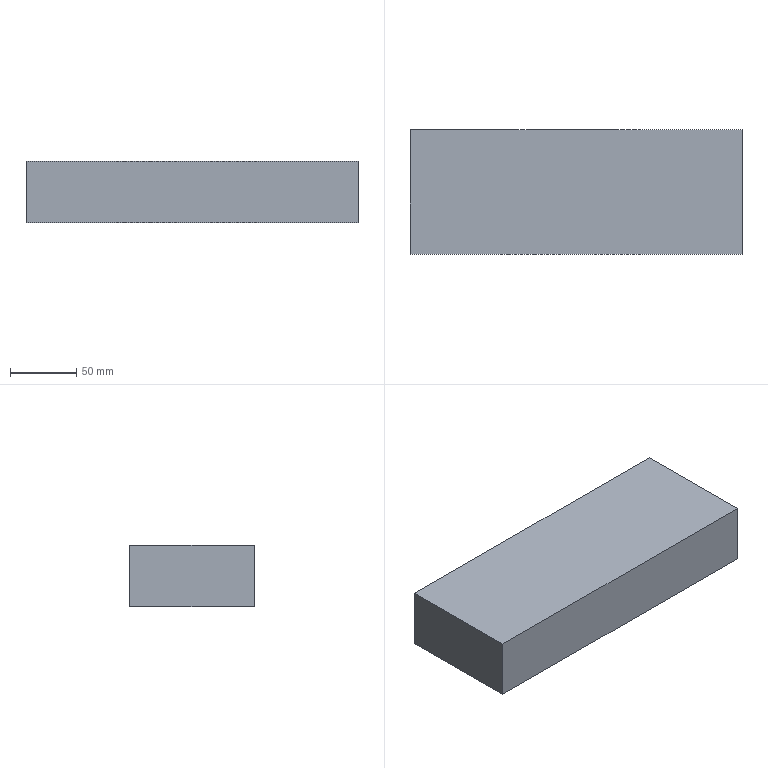Part | SolidWorks | features Extrusion 1, MoveFace 1 | 1 solid | 6 faces | box 250 x 93.801 x 46.3 mm | volume 1085747 mm3 | plane 6
STEP:
#1=CARTESIAN_POINT('',(125.,733.801,0.));
#2=VERTEX_POINT('',#1);
#3=CARTESIAN_POINT('',(125.,827.602,0.));
#4=VERTEX_POINT('',#3);
#5=CARTESIAN_POINT('',(125.,733.801,0.));
#6=DIRECTION('',(0.,1.,0.));
#7=VECTOR('',#6,1000.);
#8=LINE('',#5,#7);
#9=EDGE_CURVE('',#2,#4,#8,.T.);
#10=ORIENTED_EDGE('',*,*,#9,.T.);
#11=CARTESIAN_POINT('',(125.,827.602,46.3));
#12=VERTEX_POINT('',#11);
#13=CARTESIAN_POINT('',(125.,827.602,44.));
#14=DIRECTION('',(0.,0.,-1.));
#15=VECTOR('',#14,1000.);
#16=LINE('',#13,#15);
#17=EDGE_CURVE('',#12,#4,#16,.T.);
#18=ORIENTED_EDGE('',*,*,#17,.F.);
#19=CARTESIAN_POINT('',(125.,733.801,46.3));
#20=VERTEX_POINT('',#19);
#21=CARTESIAN_POINT('',(125.,733.801,46.3));
#22=DIRECTION('',(0.,1.,0.));
#23=VECTOR('',#22,1000.);
#24=LINE('',#21,#23);
#25=EDGE_CURVE('',#20,#12,#24,.T.);
#26=ORIENTED_EDGE('',*,*,#25,.F.);
#27=CARTESIAN_POINT('',(125.,733.801,44.));
#28=DIRECTION('',(0.,0.,-1.));
#29=VECTOR('',#28,1000.);
#30=LINE('',#27,#29);
#31=EDGE_CURVE('',#20,#2,#30,.T.);
#32=ORIENTED_EDGE('',*,*,#31,.T.);
#33=EDGE_LOOP('',(#10,#18,#26,#32));
#34=FACE_OUTER_BOUND('',#33,.T.);
#35=CARTESIAN_POINT('',(125.,733.801,44.));
#36=DIRECTION('',(-1.,0.,0.));
#37=DIRECTION('',(0.,0.,1.));
#38=AXIS2_PLACEMENT_3D('',#35,#36,#37);
#39=PLANE('',#38);
#40=ADVANCED_FACE('',(#34),#39,.F.);
#41=CARTESIAN_POINT('',(-125.,827.602,0.));
#42=VERTEX_POINT('',#41);
#43=CARTESIAN_POINT('',(125.,827.602,0.));
#44=DIRECTION('',(-1.,0.,0.));
#45=VECTOR('',#44,1000.);
#46=LINE('',#43,#45);
#47=EDGE_CURVE('',#4,#42,#46,.T.);
#48=ORIENTED_EDGE('',*,*,#47,.T.);
#49=CARTESIAN_POINT('',(-125.,827.602,46.3));
#50=VERTEX_POINT('',#49);
#51=CARTESIAN_POINT('',(-125.,827.602,44.));
#52=DIRECTION('',(0.,0.,-1.));
#53=VECTOR('',#52,1000.);
#54=LINE('',#51,#53);
#55=EDGE_CURVE('',#50,#42,#54,.T.);
#56=ORIENTED_EDGE('',*,*,#55,.F.);
#57=CARTESIAN_POINT('',(125.,827.602,46.3));
#58=DIRECTION('',(-1.,0.,0.));
#59=VECTOR('',#58,1000.);
#60=LINE('',#57,#59);
#61=EDGE_CURVE('',#12,#50,#60,.T.);
#62=ORIENTED_EDGE('',*,*,#61,.F.);
#63=ORIENTED_EDGE('',*,*,#17,.T.);
#64=EDGE_LOOP('',(#48,#56,#62,#63));
#65=FACE_OUTER_BOUND('',#64,.T.);
#66=CARTESIAN_POINT('',(125.,827.602,44.));
#67=DIRECTION('',(0.,-1.,0.));
#68=DIRECTION('',(0.,0.,-1.));
#69=AXIS2_PLACEMENT_3D('',#66,#67,#68);
#70=PLANE('',#69);
#71=ADVANCED_FACE('',(#65),#70,.F.);
#72=CARTESIAN_POINT('',(-125.,733.801,0.));
#73=VERTEX_POINT('',#72);
#74=CARTESIAN_POINT('',(-125.,733.801,0.));
#75=DIRECTION('',(0.,-1.,0.));
#76=VECTOR('',#75,1000.);
#77=LINE('',#74,#76);
#78=EDGE_CURVE('',#42,#73,#77,.T.);
#79=ORIENTED_EDGE('',*,*,#78,.T.);
#80=CARTESIAN_POINT('',(-125.,733.801,46.3));
#81=VERTEX_POINT('',#80);
#82=CARTESIAN_POINT('',(-125.,733.801,44.));
#83=DIRECTION('',(0.,0.,-1.));
#84=VECTOR('',#83,1000.);
#85=LINE('',#82,#84);
#86=EDGE_CURVE('',#81,#73,#85,.T.);
#87=ORIENTED_EDGE('',*,*,#86,.F.);
#88=CARTESIAN_POINT('',(-125.,733.801,46.3));
#89=DIRECTION('',(0.,-1.,0.));
#90=VECTOR('',#89,1000.);
#91=LINE('',#88,#90);
#92=EDGE_CURVE('',#50,#81,#91,.T.);
#93=ORIENTED_EDGE('',*,*,#92,.F.);
#94=ORIENTED_EDGE('',*,*,#55,.T.);
#95=EDGE_LOOP('',(#79,#87,#93,#94));
#96=FACE_OUTER_BOUND('',#95,.T.);
#97=CARTESIAN_POINT('',(-125.,733.801,44.));
#98=DIRECTION('',(1.,0.,0.));
#99=DIRECTION('',(0.,1.,0.));
#100=AXIS2_PLACEMENT_3D('',#97,#98,#99);
#101=PLANE('',#100);
#102=ADVANCED_FACE('',(#96),#101,.F.);
#103=CARTESIAN_POINT('',(125.,733.801,0.));
#104=DIRECTION('',(1.,0.,0.));
#105=VECTOR('',#104,1000.);
#106=LINE('',#103,#105);
#107=EDGE_CURVE('',#73,#2,#106,.T.);
#108=ORIENTED_EDGE('',*,*,#107,.T.);
#109=ORIENTED_EDGE('',*,*,#31,.F.);
#110=CARTESIAN_POINT('',(125.,733.801,46.3));
#111=DIRECTION('',(1.,0.,0.));
#112=VECTOR('',#111,1000.);
#113=LINE('',#110,#112);
#114=EDGE_CURVE('',#81,#20,#113,.T.);
#115=ORIENTED_EDGE('',*,*,#114,.F.);
#116=ORIENTED_EDGE('',*,*,#86,.T.);
#117=EDGE_LOOP('',(#108,#109,#115,#116));
#118=FACE_OUTER_BOUND('',#117,.T.);
#119=CARTESIAN_POINT('',(125.,733.801,44.));
#120=DIRECTION('',(0.,1.,0.));
#121=DIRECTION('',(0.,0.,1.));
#122=AXIS2_PLACEMENT_3D('',#119,#120,#121);
#123=PLANE('',#122);
#124=ADVANCED_FACE('',(#118),#123,.F.);
#125=ORIENTED_EDGE('',*,*,#25,.T.);
#126=ORIENTED_EDGE('',*,*,#61,.T.);
#127=ORIENTED_EDGE('',*,*,#92,.T.);
#128=ORIENTED_EDGE('',*,*,#114,.T.);
#129=EDGE_LOOP('',(#125,#126,#127,#128));
#130=FACE_OUTER_BOUND('',#129,.T.);
#131=CARTESIAN_POINT('',(0.,0.,46.3));
#132=DIRECTION('',(0.,0.,1.));
#133=DIRECTION('',(1.,0.,0.));
#134=AXIS2_PLACEMENT_3D('',#131,#132,#133);
#135=PLANE('',#134);
#136=ADVANCED_FACE('',(#130),#135,.T.);
#137=ORIENTED_EDGE('',*,*,#9,.F.);
#138=ORIENTED_EDGE('',*,*,#107,.F.);
#139=ORIENTED_EDGE('',*,*,#78,.F.);
#140=ORIENTED_EDGE('',*,*,#47,.F.);
#141=EDGE_LOOP('',(#137,#138,#139,#140));
#142=FACE_OUTER_BOUND('',#141,.T.);
#143=CARTESIAN_POINT('',(0.,0.,0.));
#144=DIRECTION('',(0.,0.,1.));
#145=DIRECTION('',(1.,0.,0.));
#146=AXIS2_PLACEMENT_3D('',#143,#144,#145);
#147=PLANE('',#146);
#148=ADVANCED_FACE('',(#142),#147,.F.);
#149=CLOSED_SHELL('',(#40,#71,#102,#124,#136,#148));
#150=MANIFOLD_SOLID_BREP('',#149);
#151=CARTESIAN_POINT('',(0.,0.,0.));
#152=DIRECTION('',(0.,0.,1.));
#153=DIRECTION('',(1.,0.,0.));
#154=AXIS2_PLACEMENT_3D('',#151,#152,#153);
#155=(LENGTH_UNIT()NAMED_UNIT(*)SI_UNIT(.MILLI.,.METRE.));
#156=UNCERTAINTY_MEASURE_WITH_UNIT(LENGTH_MEASURE(0.00001),#155,'','');
#157=(NAMED_UNIT(*)PLANE_ANGLE_UNIT()SI_UNIT($,.RADIAN.));
#158=(NAMED_UNIT(*)SI_UNIT($,.STERADIAN.)SOLID_ANGLE_UNIT());
#159=(GEOMETRIC_REPRESENTATION_CONTEXT(3)GLOBAL_UNCERTAINTY_ASSIGNED_CONTEXT((#156))GLOBAL_UNIT_ASSIGNED_CONTEXT((#155,#157,#158))REPRESENTATION_CONTEXT('',''));
#160=ADVANCED_BREP_SHAPE_REPRESENTATION('',(#150,#154),#159);